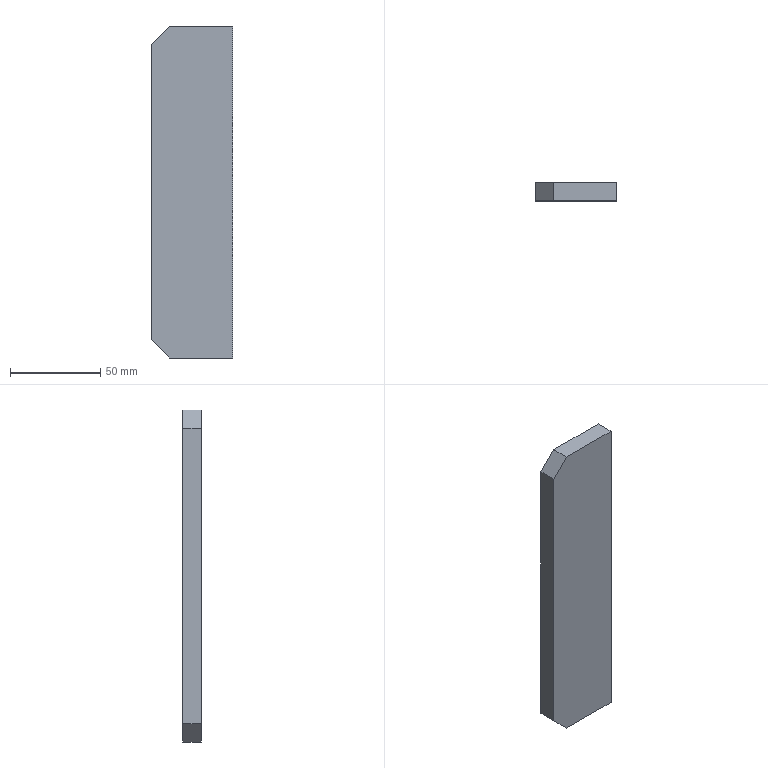Part | STEP file | Beam填充筋Plate-200×100-2 | 1 solid | 8 faces | box 45 x 10 x 184 mm | volume 81800 mm3 | plane 8
STEP:
#1=CARTESIAN_POINT('',(0.,0.,0.));
#2=DIRECTION('',(0.,0.,1.));
#3=DIRECTION('',(1.,0.,0.));
#4=AXIS2_PLACEMENT_3D('',#1,#2,#3);
#5=CARTESIAN_POINT('',(45.,0.,92.));
#6=VERTEX_POINT('',#5);
#7=CARTESIAN_POINT('',(45.,0.,-92.));
#8=VERTEX_POINT('',#7);
#9=CARTESIAN_POINT('',(45.,0.,-92.));
#10=DIRECTION('',(0.,0.,-1.));
#11=VECTOR('',#10,1.);
#12=LINE('',#9,#11);
#13=CARTESIAN_POINT('',(45.,10.,-92.));
#14=DIRECTION('',(-1.,0.,0.));
#15=DIRECTION('',(0.,0.,1.));
#16=AXIS2_PLACEMENT_3D('',#13,#14,#15);
#17=PLANE('',#16);
#18=CARTESIAN_POINT('',(0.,-10.));
#19=DIRECTION('',(-1.,0.));
#20=VECTOR('',#19,1.);
#21=LINE('',#18,#20);
#22=(GEOMETRIC_REPRESENTATION_CONTEXT(2)PARAMETRIC_REPRESENTATION_CONTEXT()REPRESENTATION_CONTEXT('',''));
#23=DEFINITIONAL_REPRESENTATION('',(#21),#22);
#24=PCURVE('',#17,#23);
#25=CARTESIAN_POINT('',(0.,0.,0.));
#26=DIRECTION('',(0.,-1.,0.));
#27=DIRECTION('',(0.,0.,-1.));
#28=AXIS2_PLACEMENT_3D('',#25,#26,#27);
#29=PLANE('',#28);
#30=CARTESIAN_POINT('',(92.,45.));
#31=DIRECTION('',(1.,0.));
#32=VECTOR('',#31,1.);
#33=LINE('',#30,#32);
#34=(GEOMETRIC_REPRESENTATION_CONTEXT(2)PARAMETRIC_REPRESENTATION_CONTEXT()REPRESENTATION_CONTEXT('',''));
#35=DEFINITIONAL_REPRESENTATION('',(#33),#34);
#36=PCURVE('',#29,#35);
#37=SURFACE_CURVE('',#12,(#24,#36),.PCURVE_S1.);
#38=EDGE_CURVE('',#6,#8,#37,.T.);
#39=ORIENTED_EDGE('',*,*,#38,.T.);
#40=CARTESIAN_POINT('',(45.,10.,-92.));
#41=VERTEX_POINT('',#40);
#42=CARTESIAN_POINT('',(45.,10.,-92.));
#43=DIRECTION('',(0.,-1.,0.));
#44=VECTOR('',#43,1.);
#45=LINE('',#42,#44);
#46=CARTESIAN_POINT('',(0.,0.));
#47=DIRECTION('',(0.,-1.));
#48=VECTOR('',#47,1.);
#49=LINE('',#46,#48);
#50=(GEOMETRIC_REPRESENTATION_CONTEXT(2)PARAMETRIC_REPRESENTATION_CONTEXT()REPRESENTATION_CONTEXT('',''));
#51=DEFINITIONAL_REPRESENTATION('',(#49),#50);
#52=PCURVE('',#17,#51);
#53=CARTESIAN_POINT('',(0.,10.,-92.));
#54=DIRECTION('',(0.,0.,1.));
#55=DIRECTION('',(1.,0.,0.));
#56=AXIS2_PLACEMENT_3D('',#53,#54,#55);
#57=PLANE('',#56);
#58=CARTESIAN_POINT('',(45.,0.));
#59=DIRECTION('',(0.,-1.));
#60=VECTOR('',#59,1.);
#61=LINE('',#58,#60);
#62=(GEOMETRIC_REPRESENTATION_CONTEXT(2)PARAMETRIC_REPRESENTATION_CONTEXT()REPRESENTATION_CONTEXT('',''));
#63=DEFINITIONAL_REPRESENTATION('',(#61),#62);
#64=PCURVE('',#57,#63);
#65=SURFACE_CURVE('',#45,(#52,#64),.PCURVE_S1.);
#66=EDGE_CURVE('',#41,#8,#65,.T.);
#67=ORIENTED_EDGE('',*,*,#66,.F.);
#68=CARTESIAN_POINT('',(45.,10.,92.));
#69=VERTEX_POINT('',#68);
#70=CARTESIAN_POINT('',(45.,10.,-92.));
#71=DIRECTION('',(0.,0.,-1.));
#72=VECTOR('',#71,1.);
#73=LINE('',#70,#72);
#74=CARTESIAN_POINT('',(0.,0.));
#75=DIRECTION('',(-1.,0.));
#76=VECTOR('',#75,1.);
#77=LINE('',#74,#76);
#78=(GEOMETRIC_REPRESENTATION_CONTEXT(2)PARAMETRIC_REPRESENTATION_CONTEXT()REPRESENTATION_CONTEXT('',''));
#79=DEFINITIONAL_REPRESENTATION('',(#77),#78);
#80=PCURVE('',#17,#79);
#81=CARTESIAN_POINT('',(0.,10.,0.));
#82=DIRECTION('',(0.,-1.,0.));
#83=DIRECTION('',(0.,0.,-1.));
#84=AXIS2_PLACEMENT_3D('',#81,#82,#83);
#85=PLANE('',#84);
#86=CARTESIAN_POINT('',(92.,45.));
#87=DIRECTION('',(1.,0.));
#88=VECTOR('',#87,1.);
#89=LINE('',#86,#88);
#90=(GEOMETRIC_REPRESENTATION_CONTEXT(2)PARAMETRIC_REPRESENTATION_CONTEXT()REPRESENTATION_CONTEXT('',''));
#91=DEFINITIONAL_REPRESENTATION('',(#89),#90);
#92=PCURVE('',#85,#91);
#93=SURFACE_CURVE('',#73,(#80,#92),.PCURVE_S1.);
#94=EDGE_CURVE('',#69,#41,#93,.T.);
#95=ORIENTED_EDGE('',*,*,#94,.F.);
#96=CARTESIAN_POINT('',(45.,10.,92.));
#97=DIRECTION('',(0.,-1.,0.));
#98=VECTOR('',#97,1.);
#99=LINE('',#96,#98);
#100=CARTESIAN_POINT('',(184.,0.));
#101=DIRECTION('',(0.,-1.));
#102=VECTOR('',#101,1.);
#103=LINE('',#100,#102);
#104=(GEOMETRIC_REPRESENTATION_CONTEXT(2)PARAMETRIC_REPRESENTATION_CONTEXT()REPRESENTATION_CONTEXT('',''));
#105=DEFINITIONAL_REPRESENTATION('',(#103),#104);
#106=PCURVE('',#17,#105);
#107=CARTESIAN_POINT('',(45.,10.,92.));
#108=DIRECTION('',(0.,0.,-1.));
#109=DIRECTION('',(-1.,0.,0.));
#110=AXIS2_PLACEMENT_3D('',#107,#108,#109);
#111=PLANE('',#110);
#112=CARTESIAN_POINT('',(0.,0.));
#113=DIRECTION('',(0.,-1.));
#114=VECTOR('',#113,1.);
#115=LINE('',#112,#114);
#116=(GEOMETRIC_REPRESENTATION_CONTEXT(2)PARAMETRIC_REPRESENTATION_CONTEXT()REPRESENTATION_CONTEXT('',''));
#117=DEFINITIONAL_REPRESENTATION('',(#115),#116);
#118=PCURVE('',#111,#117);
#119=SURFACE_CURVE('',#99,(#106,#118),.PCURVE_S1.);
#120=EDGE_CURVE('',#69,#6,#119,.T.);
#121=ORIENTED_EDGE('',*,*,#120,.T.);
#122=EDGE_LOOP('',(#39,#67,#95,#121));
#123=FACE_BOUND('',#122,.T.);
#124=ADVANCED_FACE('',(#123),#17,.F.);
#125=CARTESIAN_POINT('',(10.,0.,-92.));
#126=VERTEX_POINT('',#125);
#127=CARTESIAN_POINT('',(0.,0.,-92.));
#128=DIRECTION('',(-1.,0.,0.));
#129=VECTOR('',#128,1.);
#130=LINE('',#127,#129);
#131=CARTESIAN_POINT('',(0.,-10.));
#132=DIRECTION('',(-1.,0.));
#133=VECTOR('',#132,1.);
#134=LINE('',#131,#133);
#135=(GEOMETRIC_REPRESENTATION_CONTEXT(2)PARAMETRIC_REPRESENTATION_CONTEXT()REPRESENTATION_CONTEXT('',''));
#136=DEFINITIONAL_REPRESENTATION('',(#134),#135);
#137=PCURVE('',#57,#136);
#138=CARTESIAN_POINT('',(92.,0.));
#139=DIRECTION('',(0.,-1.));
#140=VECTOR('',#139,1.);
#141=LINE('',#138,#140);
#142=(GEOMETRIC_REPRESENTATION_CONTEXT(2)PARAMETRIC_REPRESENTATION_CONTEXT()REPRESENTATION_CONTEXT('',''));
#143=DEFINITIONAL_REPRESENTATION('',(#141),#142);
#144=PCURVE('',#29,#143);
#145=SURFACE_CURVE('',#130,(#137,#144),.PCURVE_S1.);
#146=EDGE_CURVE('',#8,#126,#145,.T.);
#147=ORIENTED_EDGE('',*,*,#146,.T.);
#148=CARTESIAN_POINT('',(10.,10.,-92.));
#149=VERTEX_POINT('',#148);
#150=CARTESIAN_POINT('',(10.,10.,-92.));
#151=DIRECTION('',(0.,1.,0.));
#152=VECTOR('',#151,1.);
#153=LINE('',#150,#152);
#154=CARTESIAN_POINT('',(10.,0.));
#155=DIRECTION('',(0.,1.));
#156=VECTOR('',#155,1.);
#157=LINE('',#154,#156);
#158=(GEOMETRIC_REPRESENTATION_CONTEXT(2)PARAMETRIC_REPRESENTATION_CONTEXT()REPRESENTATION_CONTEXT('',''));
#159=DEFINITIONAL_REPRESENTATION('',(#157),#158);
#160=PCURVE('',#57,#159);
#161=CARTESIAN_POINT('',(0.,10.,-82.));
#162=DIRECTION('',(0.7071,0.,0.7071));
#163=DIRECTION('',(0.,-1.,0.));
#164=AXIS2_PLACEMENT_3D('',#161,#162,#163);
#165=PLANE('',#164);
#166=CARTESIAN_POINT('',(0.,14.142));
#167=DIRECTION('',(-1.,0.));
#168=VECTOR('',#167,1.);
#169=LINE('',#166,#168);
#170=(GEOMETRIC_REPRESENTATION_CONTEXT(2)PARAMETRIC_REPRESENTATION_CONTEXT()REPRESENTATION_CONTEXT('',''));
#171=DEFINITIONAL_REPRESENTATION('',(#169),#170);
#172=PCURVE('',#165,#171);
#173=SURFACE_CURVE('',#153,(#160,#172),.PCURVE_S1.);
#174=EDGE_CURVE('',#126,#149,#173,.T.);
#175=ORIENTED_EDGE('',*,*,#174,.T.);
#176=CARTESIAN_POINT('',(0.,10.,-92.));
#177=DIRECTION('',(-1.,0.,0.));
#178=VECTOR('',#177,1.);
#179=LINE('',#176,#178);
#180=CARTESIAN_POINT('',(0.,0.));
#181=DIRECTION('',(-1.,0.));
#182=VECTOR('',#181,1.);
#183=LINE('',#180,#182);
#184=(GEOMETRIC_REPRESENTATION_CONTEXT(2)PARAMETRIC_REPRESENTATION_CONTEXT()REPRESENTATION_CONTEXT('',''));
#185=DEFINITIONAL_REPRESENTATION('',(#183),#184);
#186=PCURVE('',#57,#185);
#187=CARTESIAN_POINT('',(92.,0.));
#188=DIRECTION('',(0.,-1.));
#189=VECTOR('',#188,1.);
#190=LINE('',#187,#189);
#191=(GEOMETRIC_REPRESENTATION_CONTEXT(2)PARAMETRIC_REPRESENTATION_CONTEXT()REPRESENTATION_CONTEXT('',''));
#192=DEFINITIONAL_REPRESENTATION('',(#190),#191);
#193=PCURVE('',#85,#192);
#194=SURFACE_CURVE('',#179,(#186,#193),.PCURVE_S1.);
#195=EDGE_CURVE('',#41,#149,#194,.T.);
#196=ORIENTED_EDGE('',*,*,#195,.F.);
#197=ORIENTED_EDGE('',*,*,#66,.T.);
#198=EDGE_LOOP('',(#147,#175,#196,#197));
#199=FACE_BOUND('',#198,.T.);
#200=ADVANCED_FACE('',(#199),#57,.F.);
#201=CARTESIAN_POINT('',(0.,0.,-82.));
#202=VERTEX_POINT('',#201);
#203=CARTESIAN_POINT('',(0.,0.,82.));
#204=VERTEX_POINT('',#203);
#205=CARTESIAN_POINT('',(0.,0.,92.));
#206=DIRECTION('',(0.,0.,1.));
#207=VECTOR('',#206,1.);
#208=LINE('',#205,#207);
#209=CARTESIAN_POINT('',(0.,10.,92.));
#210=DIRECTION('',(1.,0.,0.));
#211=DIRECTION('',(0.,0.,-1.));
#212=AXIS2_PLACEMENT_3D('',#209,#210,#211);
#213=PLANE('',#212);
#214=CARTESIAN_POINT('',(0.,-10.));
#215=DIRECTION('',(-1.,0.));
#216=VECTOR('',#215,1.);
#217=LINE('',#214,#216);
#218=(GEOMETRIC_REPRESENTATION_CONTEXT(2)PARAMETRIC_REPRESENTATION_CONTEXT()REPRESENTATION_CONTEXT('',''));
#219=DEFINITIONAL_REPRESENTATION('',(#217),#218);
#220=PCURVE('',#213,#219);
#221=CARTESIAN_POINT('',(-92.,0.));
#222=DIRECTION('',(-1.,0.));
#223=VECTOR('',#222,1.);
#224=LINE('',#221,#223);
#225=(GEOMETRIC_REPRESENTATION_CONTEXT(2)PARAMETRIC_REPRESENTATION_CONTEXT()REPRESENTATION_CONTEXT('',''));
#226=DEFINITIONAL_REPRESENTATION('',(#224),#225);
#227=PCURVE('',#29,#226);
#228=SURFACE_CURVE('',#208,(#220,#227),.PCURVE_S1.);
#229=EDGE_CURVE('',#202,#204,#228,.T.);
#230=ORIENTED_EDGE('',*,*,#229,.T.);
#231=CARTESIAN_POINT('',(0.,10.,82.));
#232=VERTEX_POINT('',#231);
#233=CARTESIAN_POINT('',(0.,10.,82.));
#234=DIRECTION('',(0.,1.,0.));
#235=VECTOR('',#234,1.);
#236=LINE('',#233,#235);
#237=CARTESIAN_POINT('',(10.,0.));
#238=DIRECTION('',(0.,1.));
#239=VECTOR('',#238,1.);
#240=LINE('',#237,#239);
#241=(GEOMETRIC_REPRESENTATION_CONTEXT(2)PARAMETRIC_REPRESENTATION_CONTEXT()REPRESENTATION_CONTEXT('',''));
#242=DEFINITIONAL_REPRESENTATION('',(#240),#241);
#243=PCURVE('',#213,#242);
#244=CARTESIAN_POINT('',(10.,10.,92.));
#245=DIRECTION('',(0.7071,0.,-0.7071));
#246=DIRECTION('',(0.,-1.,0.));
#247=AXIS2_PLACEMENT_3D('',#244,#245,#246);
#248=PLANE('',#247);
#249=CARTESIAN_POINT('',(0.,14.142));
#250=DIRECTION('',(-1.,0.));
#251=VECTOR('',#250,1.);
#252=LINE('',#249,#251);
#253=(GEOMETRIC_REPRESENTATION_CONTEXT(2)PARAMETRIC_REPRESENTATION_CONTEXT()REPRESENTATION_CONTEXT('',''));
#254=DEFINITIONAL_REPRESENTATION('',(#252),#253);
#255=PCURVE('',#248,#254);
#256=SURFACE_CURVE('',#236,(#243,#255),.PCURVE_S1.);
#257=EDGE_CURVE('',#204,#232,#256,.T.);
#258=ORIENTED_EDGE('',*,*,#257,.T.);
#259=CARTESIAN_POINT('',(0.,10.,-82.));
#260=VERTEX_POINT('',#259);
#261=CARTESIAN_POINT('',(0.,10.,92.));
#262=DIRECTION('',(0.,0.,1.));
#263=VECTOR('',#262,1.);
#264=LINE('',#261,#263);
#265=CARTESIAN_POINT('',(0.,0.));
#266=DIRECTION('',(-1.,0.));
#267=VECTOR('',#266,1.);
#268=LINE('',#265,#267);
#269=(GEOMETRIC_REPRESENTATION_CONTEXT(2)PARAMETRIC_REPRESENTATION_CONTEXT()REPRESENTATION_CONTEXT('',''));
#270=DEFINITIONAL_REPRESENTATION('',(#268),#269);
#271=PCURVE('',#213,#270);
#272=CARTESIAN_POINT('',(-92.,0.));
#273=DIRECTION('',(-1.,0.));
#274=VECTOR('',#273,1.);
#275=LINE('',#272,#274);
#276=(GEOMETRIC_REPRESENTATION_CONTEXT(2)PARAMETRIC_REPRESENTATION_CONTEXT()REPRESENTATION_CONTEXT('',''));
#277=DEFINITIONAL_REPRESENTATION('',(#275),#276);
#278=PCURVE('',#85,#277);
#279=SURFACE_CURVE('',#264,(#271,#278),.PCURVE_S1.);
#280=EDGE_CURVE('',#260,#232,#279,.T.);
#281=ORIENTED_EDGE('',*,*,#280,.F.);
#282=CARTESIAN_POINT('',(0.,10.,-82.));
#283=DIRECTION('',(0.,-1.,0.));
#284=VECTOR('',#283,1.);
#285=LINE('',#282,#284);
#286=CARTESIAN_POINT('',(174.,0.));
#287=DIRECTION('',(0.,-1.));
#288=VECTOR('',#287,1.);
#289=LINE('',#286,#288);
#290=(GEOMETRIC_REPRESENTATION_CONTEXT(2)PARAMETRIC_REPRESENTATION_CONTEXT()REPRESENTATION_CONTEXT('',''));
#291=DEFINITIONAL_REPRESENTATION('',(#289),#290);
#292=PCURVE('',#213,#291);
#293=CARTESIAN_POINT('',(0.,0.));
#294=DIRECTION('',(1.,0.));
#295=VECTOR('',#294,1.);
#296=LINE('',#293,#295);
#297=(GEOMETRIC_REPRESENTATION_CONTEXT(2)PARAMETRIC_REPRESENTATION_CONTEXT()REPRESENTATION_CONTEXT('',''));
#298=DEFINITIONAL_REPRESENTATION('',(#296),#297);
#299=PCURVE('',#165,#298);
#300=SURFACE_CURVE('',#285,(#292,#299),.PCURVE_S1.);
#301=EDGE_CURVE('',#260,#202,#300,.T.);
#302=ORIENTED_EDGE('',*,*,#301,.T.);
#303=EDGE_LOOP('',(#230,#258,#281,#302));
#304=FACE_BOUND('',#303,.T.);
#305=ADVANCED_FACE('',(#304),#213,.F.);
#306=CARTESIAN_POINT('',(10.,10.,92.));
#307=VERTEX_POINT('',#306);
#308=CARTESIAN_POINT('',(45.,10.,92.));
#309=DIRECTION('',(1.,0.,0.));
#310=VECTOR('',#309,1.);
#311=LINE('',#308,#310);
#312=CARTESIAN_POINT('',(0.,0.));
#313=DIRECTION('',(-1.,0.));
#314=VECTOR('',#313,1.);
#315=LINE('',#312,#314);
#316=(GEOMETRIC_REPRESENTATION_CONTEXT(2)PARAMETRIC_REPRESENTATION_CONTEXT()REPRESENTATION_CONTEXT('',''));
#317=DEFINITIONAL_REPRESENTATION('',(#315),#316);
#318=PCURVE('',#111,#317);
#319=CARTESIAN_POINT('',(-92.,45.));
#320=DIRECTION('',(0.,1.));
#321=VECTOR('',#320,1.);
#322=LINE('',#319,#321);
#323=(GEOMETRIC_REPRESENTATION_CONTEXT(2)PARAMETRIC_REPRESENTATION_CONTEXT()REPRESENTATION_CONTEXT('',''));
#324=DEFINITIONAL_REPRESENTATION('',(#322),#323);
#325=PCURVE('',#85,#324);
#326=SURFACE_CURVE('',#311,(#318,#325),.PCURVE_S1.);
#327=EDGE_CURVE('',#307,#69,#326,.T.);
#328=ORIENTED_EDGE('',*,*,#327,.F.);
#329=CARTESIAN_POINT('',(10.,0.,92.));
#330=VERTEX_POINT('',#329);
#331=CARTESIAN_POINT('',(10.,10.,92.));
#332=DIRECTION('',(0.,-1.,0.));
#333=VECTOR('',#332,1.);
#334=LINE('',#331,#333);
#335=CARTESIAN_POINT('',(35.,0.));
#336=DIRECTION('',(0.,-1.));
#337=VECTOR('',#336,1.);
#338=LINE('',#335,#337);
#339=(GEOMETRIC_REPRESENTATION_CONTEXT(2)PARAMETRIC_REPRESENTATION_CONTEXT()REPRESENTATION_CONTEXT('',''));
#340=DEFINITIONAL_REPRESENTATION('',(#338),#339);
#341=PCURVE('',#111,#340);
#342=CARTESIAN_POINT('',(0.,0.));
#343=DIRECTION('',(1.,0.));
#344=VECTOR('',#343,1.);
#345=LINE('',#342,#344);
#346=(GEOMETRIC_REPRESENTATION_CONTEXT(2)PARAMETRIC_REPRESENTATION_CONTEXT()REPRESENTATION_CONTEXT('',''));
#347=DEFINITIONAL_REPRESENTATION('',(#345),#346);
#348=PCURVE('',#248,#347);
#349=SURFACE_CURVE('',#334,(#341,#348),.PCURVE_S1.);
#350=EDGE_CURVE('',#307,#330,#349,.T.);
#351=ORIENTED_EDGE('',*,*,#350,.T.);
#352=CARTESIAN_POINT('',(45.,0.,92.));
#353=DIRECTION('',(1.,0.,0.));
#354=VECTOR('',#353,1.);
#355=LINE('',#352,#354);
#356=CARTESIAN_POINT('',(0.,-10.));
#357=DIRECTION('',(-1.,0.));
#358=VECTOR('',#357,1.);
#359=LINE('',#356,#358);
#360=(GEOMETRIC_REPRESENTATION_CONTEXT(2)PARAMETRIC_REPRESENTATION_CONTEXT()REPRESENTATION_CONTEXT('',''));
#361=DEFINITIONAL_REPRESENTATION('',(#359),#360);
#362=PCURVE('',#111,#361);
#363=CARTESIAN_POINT('',(-92.,45.));
#364=DIRECTION('',(0.,1.));
#365=VECTOR('',#364,1.);
#366=LINE('',#363,#365);
#367=(GEOMETRIC_REPRESENTATION_CONTEXT(2)PARAMETRIC_REPRESENTATION_CONTEXT()REPRESENTATION_CONTEXT('',''));
#368=DEFINITIONAL_REPRESENTATION('',(#366),#367);
#369=PCURVE('',#29,#368);
#370=SURFACE_CURVE('',#355,(#362,#369),.PCURVE_S1.);
#371=EDGE_CURVE('',#330,#6,#370,.T.);
#372=ORIENTED_EDGE('',*,*,#371,.T.);
#373=ORIENTED_EDGE('',*,*,#120,.F.);
#374=EDGE_LOOP('',(#328,#351,#372,#373));
#375=FACE_BOUND('',#374,.T.);
#376=ADVANCED_FACE('',(#375),#111,.F.);
#377=ORIENTED_EDGE('',*,*,#280,.T.);
#378=CARTESIAN_POINT('',(10.,10.,92.));
#379=DIRECTION('',(0.7071,0.,0.7071));
#380=VECTOR('',#379,1.);
#381=LINE('',#378,#380);
#382=CARTESIAN_POINT('',(-92.,10.));
#383=DIRECTION('',(-0.7071,0.7071));
#384=VECTOR('',#383,1.);
#385=LINE('',#382,#384);
#386=(GEOMETRIC_REPRESENTATION_CONTEXT(2)PARAMETRIC_REPRESENTATION_CONTEXT()REPRESENTATION_CONTEXT('',''));
#387=DEFINITIONAL_REPRESENTATION('',(#385),#386);
#388=PCURVE('',#85,#387);
#389=CARTESIAN_POINT('',(0.,0.));
#390=DIRECTION('',(0.,-1.));
#391=VECTOR('',#390,1.);
#392=LINE('',#389,#391);
#393=(GEOMETRIC_REPRESENTATION_CONTEXT(2)PARAMETRIC_REPRESENTATION_CONTEXT()REPRESENTATION_CONTEXT('',''));
#394=DEFINITIONAL_REPRESENTATION('',(#392),#393);
#395=PCURVE('',#248,#394);
#396=SURFACE_CURVE('',#381,(#388,#395),.PCURVE_S1.);
#397=EDGE_CURVE('',#232,#307,#396,.T.);
#398=ORIENTED_EDGE('',*,*,#397,.T.);
#399=ORIENTED_EDGE('',*,*,#327,.T.);
#400=ORIENTED_EDGE('',*,*,#94,.T.);
#401=ORIENTED_EDGE('',*,*,#195,.T.);
#402=CARTESIAN_POINT('',(0.,10.,-82.));
#403=DIRECTION('',(-0.7071,0.,0.7071));
#404=VECTOR('',#403,1.);
#405=LINE('',#402,#404);
#406=CARTESIAN_POINT('',(82.,0.));
#407=DIRECTION('',(-0.7071,-0.7071));
#408=VECTOR('',#407,1.);
#409=LINE('',#406,#408);
#410=(GEOMETRIC_REPRESENTATION_CONTEXT(2)PARAMETRIC_REPRESENTATION_CONTEXT()REPRESENTATION_CONTEXT('',''));
#411=DEFINITIONAL_REPRESENTATION('',(#409),#410);
#412=PCURVE('',#85,#411);
#413=CARTESIAN_POINT('',(0.,0.));
#414=DIRECTION('',(0.,-1.));
#415=VECTOR('',#414,1.);
#416=LINE('',#413,#415);
#417=(GEOMETRIC_REPRESENTATION_CONTEXT(2)PARAMETRIC_REPRESENTATION_CONTEXT()REPRESENTATION_CONTEXT('',''));
#418=DEFINITIONAL_REPRESENTATION('',(#416),#417);
#419=PCURVE('',#165,#418);
#420=SURFACE_CURVE('',#405,(#412,#419),.PCURVE_S1.);
#421=EDGE_CURVE('',#149,#260,#420,.T.);
#422=ORIENTED_EDGE('',*,*,#421,.T.);
#423=EDGE_LOOP('',(#377,#398,#399,#400,#401,#422));
#424=FACE_BOUND('',#423,.T.);
#425=ADVANCED_FACE('',(#424),#85,.F.);
#426=ORIENTED_EDGE('',*,*,#371,.F.);
#427=CARTESIAN_POINT('',(-41.,0.,41.));
#428=DIRECTION('',(-0.7071,0.,-0.7071));
#429=VECTOR('',#428,1.);
#430=LINE('',#427,#429);
#431=CARTESIAN_POINT('',(-41.,-41.));
#432=DIRECTION('',(0.7071,-0.7071));
#433=VECTOR('',#432,1.);
#434=LINE('',#431,#433);
#435=(GEOMETRIC_REPRESENTATION_CONTEXT(2)PARAMETRIC_REPRESENTATION_CONTEXT()REPRESENTATION_CONTEXT('',''));
#436=DEFINITIONAL_REPRESENTATION('',(#434),#435);
#437=PCURVE('',#29,#436);
#438=CARTESIAN_POINT('',(10.,72.125));
#439=DIRECTION('',(0.,1.));
#440=VECTOR('',#439,1.);
#441=LINE('',#438,#440);
#442=(GEOMETRIC_REPRESENTATION_CONTEXT(2)PARAMETRIC_REPRESENTATION_CONTEXT()REPRESENTATION_CONTEXT('',''));
#443=DEFINITIONAL_REPRESENTATION('',(#441),#442);
#444=PCURVE('',#248,#443);
#445=SURFACE_CURVE('',#430,(#437,#444),.PCURVE_S1.);
#446=EDGE_CURVE('',#330,#204,#445,.T.);
#447=ORIENTED_EDGE('',*,*,#446,.T.);
#448=ORIENTED_EDGE('',*,*,#229,.F.);
#449=CARTESIAN_POINT('',(-41.,0.,-41.));
#450=DIRECTION('',(0.7071,0.,-0.7071));
#451=VECTOR('',#450,1.);
#452=LINE('',#449,#451);
#453=CARTESIAN_POINT('',(41.,-41.));
#454=DIRECTION('',(0.7071,0.7071));
#455=VECTOR('',#454,1.);
#456=LINE('',#453,#455);
#457=(GEOMETRIC_REPRESENTATION_CONTEXT(2)PARAMETRIC_REPRESENTATION_CONTEXT()REPRESENTATION_CONTEXT('',''));
#458=DEFINITIONAL_REPRESENTATION('',(#456),#457);
#459=PCURVE('',#29,#458);
#460=CARTESIAN_POINT('',(10.,-57.983));
#461=DIRECTION('',(0.,1.));
#462=VECTOR('',#461,1.);
#463=LINE('',#460,#462);
#464=(GEOMETRIC_REPRESENTATION_CONTEXT(2)PARAMETRIC_REPRESENTATION_CONTEXT()REPRESENTATION_CONTEXT('',''));
#465=DEFINITIONAL_REPRESENTATION('',(#463),#464);
#466=PCURVE('',#165,#465);
#467=SURFACE_CURVE('',#452,(#459,#466),.PCURVE_S1.);
#468=EDGE_CURVE('',#202,#126,#467,.T.);
#469=ORIENTED_EDGE('',*,*,#468,.T.);
#470=ORIENTED_EDGE('',*,*,#146,.F.);
#471=ORIENTED_EDGE('',*,*,#38,.F.);
#472=EDGE_LOOP('',(#426,#447,#448,#469,#470,#471));
#473=FACE_BOUND('',#472,.T.);
#474=ADVANCED_FACE('',(#473),#29,.T.);
#475=ORIENTED_EDGE('',*,*,#397,.F.);
#476=ORIENTED_EDGE('',*,*,#257,.F.);
#477=ORIENTED_EDGE('',*,*,#446,.F.);
#478=ORIENTED_EDGE('',*,*,#350,.F.);
#479=EDGE_LOOP('',(#475,#476,#477,#478));
#480=FACE_BOUND('',#479,.T.);
#481=ADVANCED_FACE('',(#480),#248,.F.);
#482=ORIENTED_EDGE('',*,*,#421,.F.);
#483=ORIENTED_EDGE('',*,*,#174,.F.);
#484=ORIENTED_EDGE('',*,*,#468,.F.);
#485=ORIENTED_EDGE('',*,*,#301,.F.);
#486=EDGE_LOOP('',(#482,#483,#484,#485));
#487=FACE_BOUND('',#486,.T.);
#488=ADVANCED_FACE('',(#487),#165,.F.);
#489=CLOSED_SHELL('',(#124,#200,#305,#376,#425,#474,#481,#488));
#490=MANIFOLD_SOLID_BREP('',#489);
#491=(LENGTH_UNIT()NAMED_UNIT(*)SI_UNIT(.MILLI.,.METRE.));
#492=UNCERTAINTY_MEASURE_WITH_UNIT(LENGTH_MEASURE(0.0000001),#491,'','');
#493=(NAMED_UNIT(*)PLANE_ANGLE_UNIT()SI_UNIT($,.RADIAN.));
#494=(NAMED_UNIT(*)SI_UNIT($,.STERADIAN.)SOLID_ANGLE_UNIT());
#495=(GEOMETRIC_REPRESENTATION_CONTEXT(3)GLOBAL_UNCERTAINTY_ASSIGNED_CONTEXT((#492))GLOBAL_UNIT_ASSIGNED_CONTEXT((#491,#493,#494))REPRESENTATION_CONTEXT('',''));
#496=ADVANCED_BREP_SHAPE_REPRESENTATION('',(#4,#490),#495);